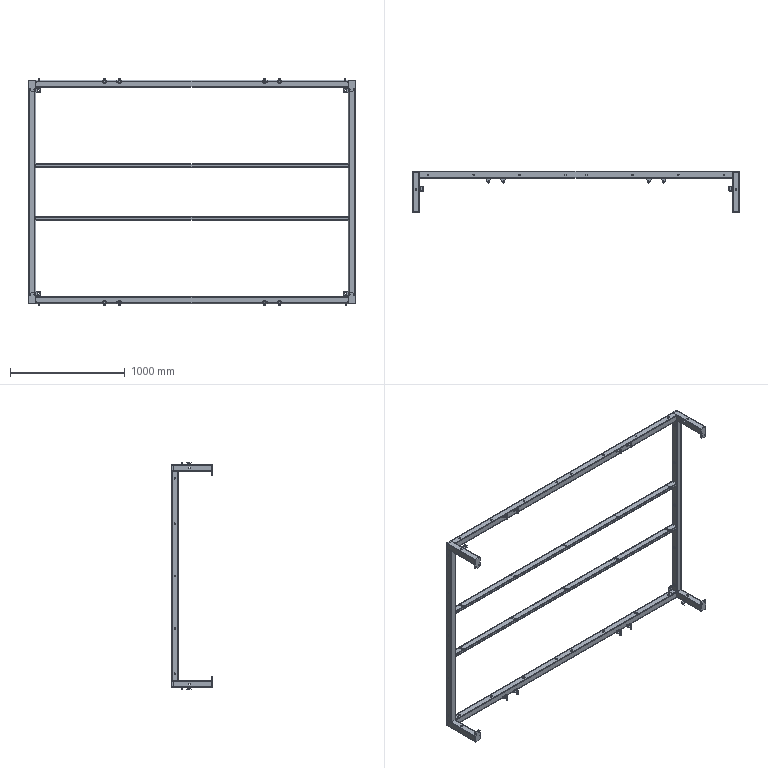Part | SolidWorks | features BaseBody 47 | 47 solids | 1395 faces | box 2850 x 360 x 1986 mm | volume 11675407 mm3 | cylinder 656 | plane 643 | cone 96 | commonest cylinder face diameters 14 x162 7 x154 6 x140 12 x48 4 x32 10 x32